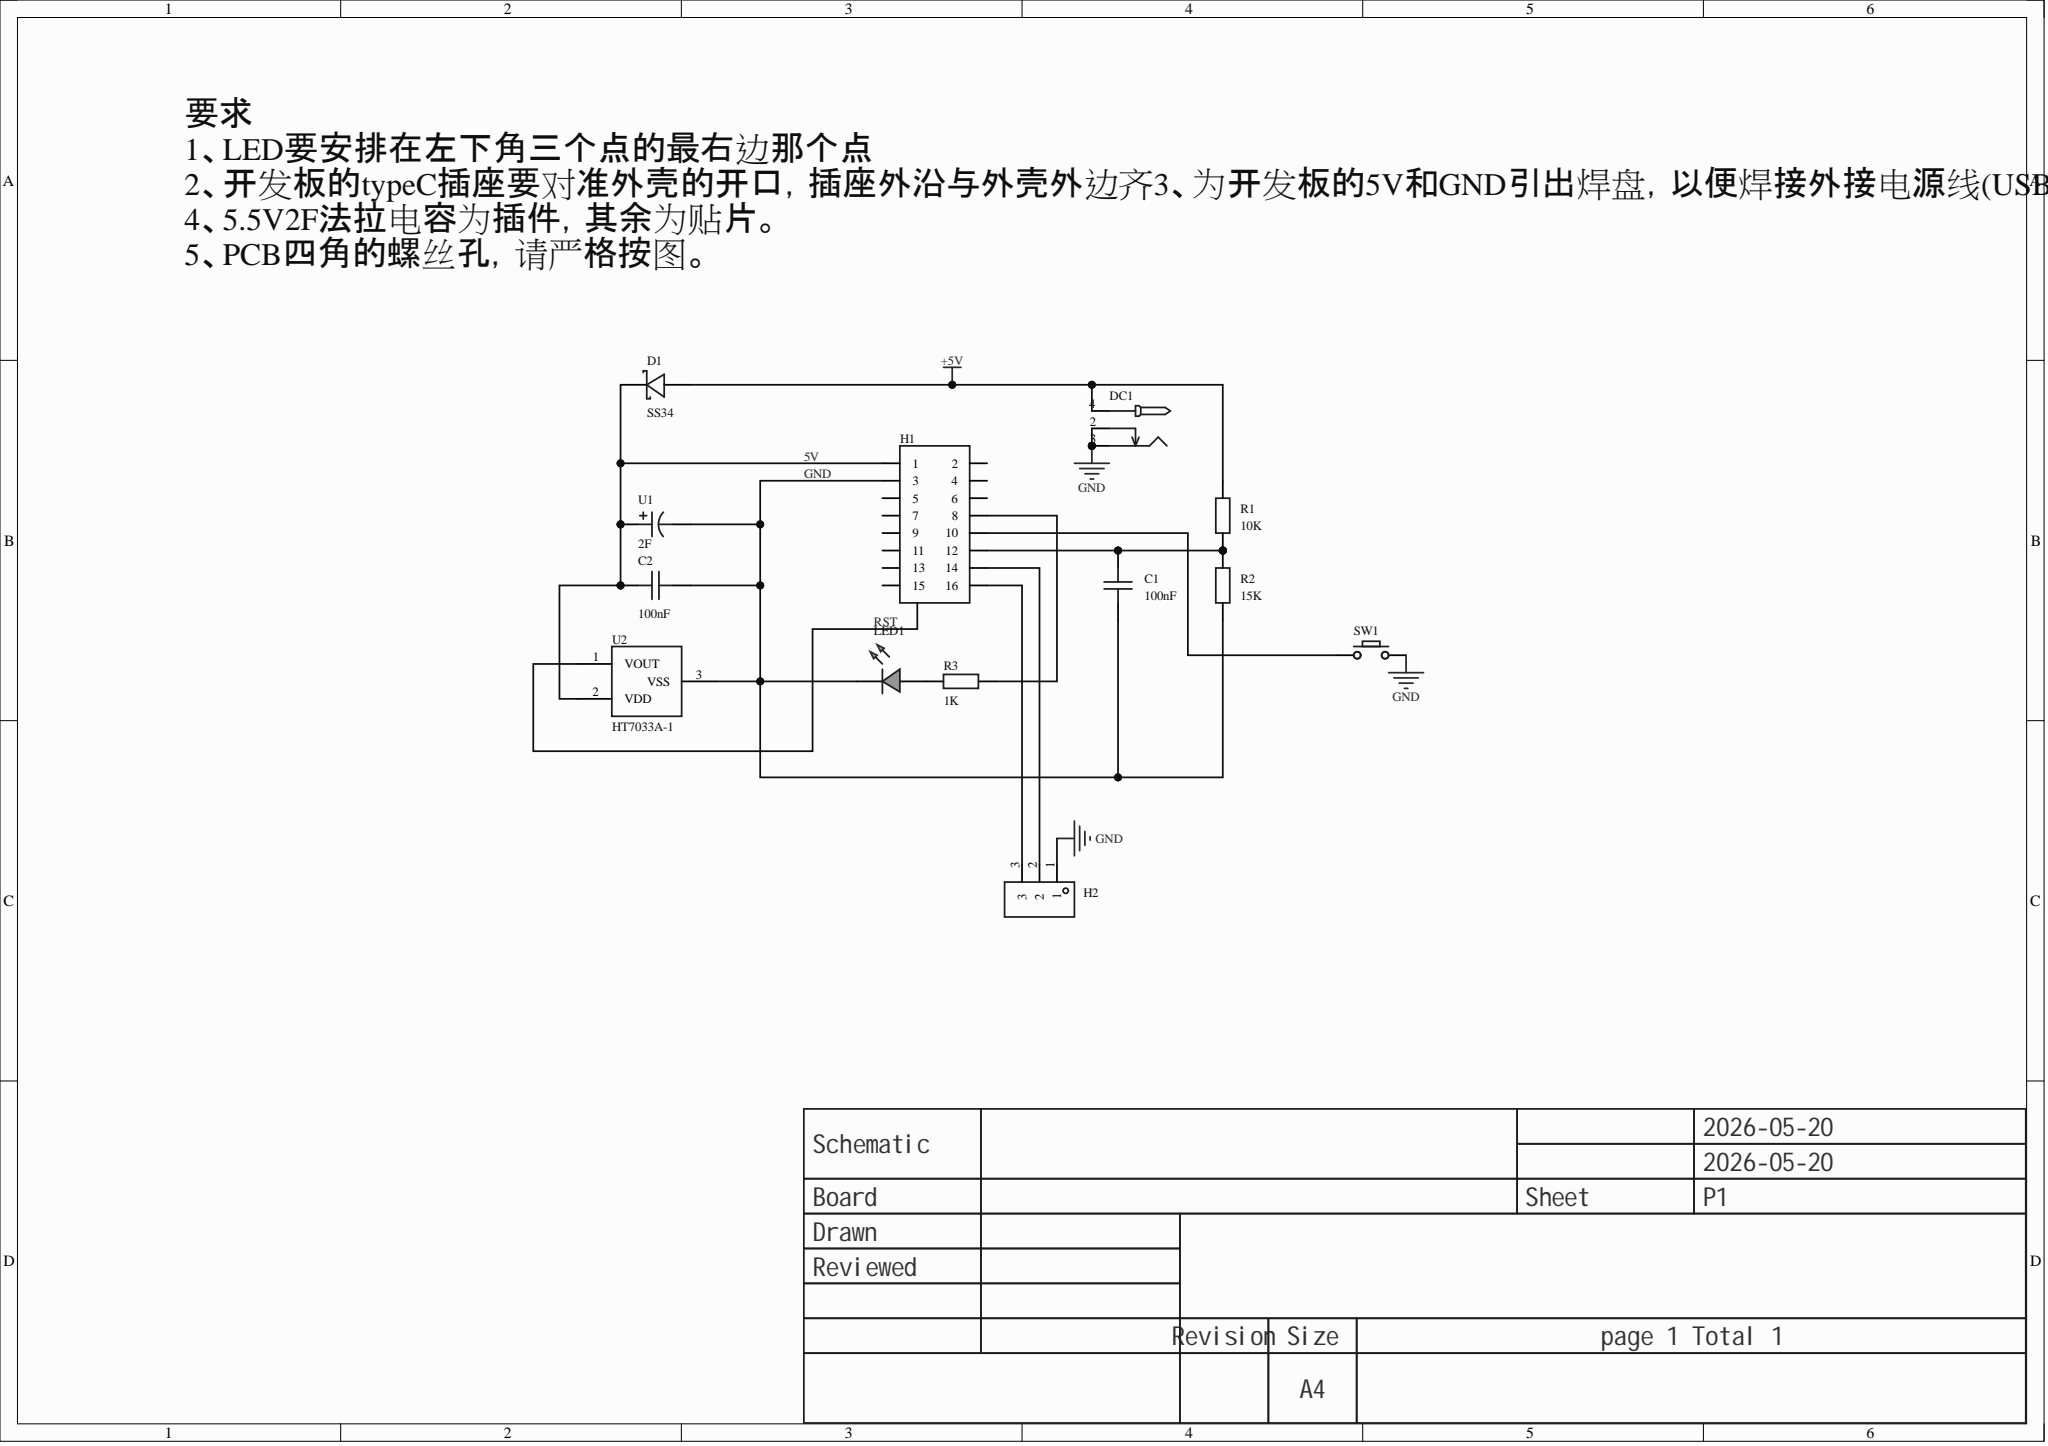Circuit board | Altium Designer | 13 parts | 9 nets
Bill of materials:
Comment,Description,Designator,Footprint,LibRef,Quantity
"100nF","","C1, C2","C0603","CAP_0603","2"
"SS34","Diode configuration:Single;Forward voltage(Vf):550mV@3A;Reverse voltage(Vr):40V;Rectified current:3A;","D1","SMA_L4.3-W2.6-LS5.2-RD","SS34_C8678","1"
"","","DC1","DC-2.0","DC-005_2.0","1"
"","","H1","HDR-TH_16P-P2.54-V-F-R2-C8-S2.54-1","HDR-F_2.54_2x8","1"
"","","H2","HDR-TH_3P-P2.54-V-M","HDR-M_2.54_1x3P","1"
"","","LED1","LED_0603","LED_0603-G","1"
"10K","","R1","R0603","Res_0603","1"
"15K","","R2","R0603","Res_0603","1"
"1K","","R3","R0603","Res_0603","1"
"","","SW1","Key_TH_3.5x6x4.3","Key_TH_3.5x6x4.3","1"
"2F","Capacitance:2F;Tolerance:-20%~+50%;Rated voltage:2.7V;Leakage current:10uA@72hrs;ESR:100mO@1kHz;","U1","CAP-TH_BD8.0-P3.50-D0.6-FD_GDC02R7R205LD0816","GDC02R7R205LD0816","1"
"HT7033A-1","Operating voltage:1.5V~30V;Reset active level:Active low;Monitored voltage count:1;Reset timeout:200us;","U2","SOT-89-3_L4.5-W2.5-P1.50-LS4.2-BR","HT7033A-1_C73715","1"
Netlist (Protel format):
[
C1
C0603
100nF



]
[
C2
C0603
100nF



]
[
D1
SMA_L4.3-W2.6-LS5.2-RD
SS34



]
[
DC1
DC-2.0




]
[
H1
HDR-TH_16P-P2.54-V-F-R2-C8-S2.54-1




]
[
H2
HDR-TH_3P-P2.54-V-M




]
[
LED1
LED_0603




]
[
R1
R0603
10K



]
[
R2
R0603
15K



]
[
R3
R0603
1K



]
[
SW1
Key_TH_3.5x6x4.3




]
[
U1
CAP-TH_BD8.0-P3.50-D0.6-FD_GDC02R7R205LD0816
2F



]
[
U2
SOT-89-3_L4.5-W2.5-P1.50-LS4.2-BR
HT7033A-1



]
(
NetLED1_2
LED1-2
R3-2
)
(
NetH1_16
H1-16
H2-3
)
(
NetH1_14
H1-14
H2-2
)
(
NetH1_10
H1-10
SW1-A
)
(
NetH1_8
H1-8
R3-1
)
(
NetC1_2
C1-2
H1-12
R1-1
R2-2
)
(
GND
C1-1
C2-1
DC1-2
DC1-3
H1-3
H2-1
LED1-1
R2-1
SW1-B
U1-2
U2-3
)
(
+5V
D1-2
DC1-4
R1-2
)
(
5V
C2-2
D1-1
H1-1
U1-1
U2-2
)